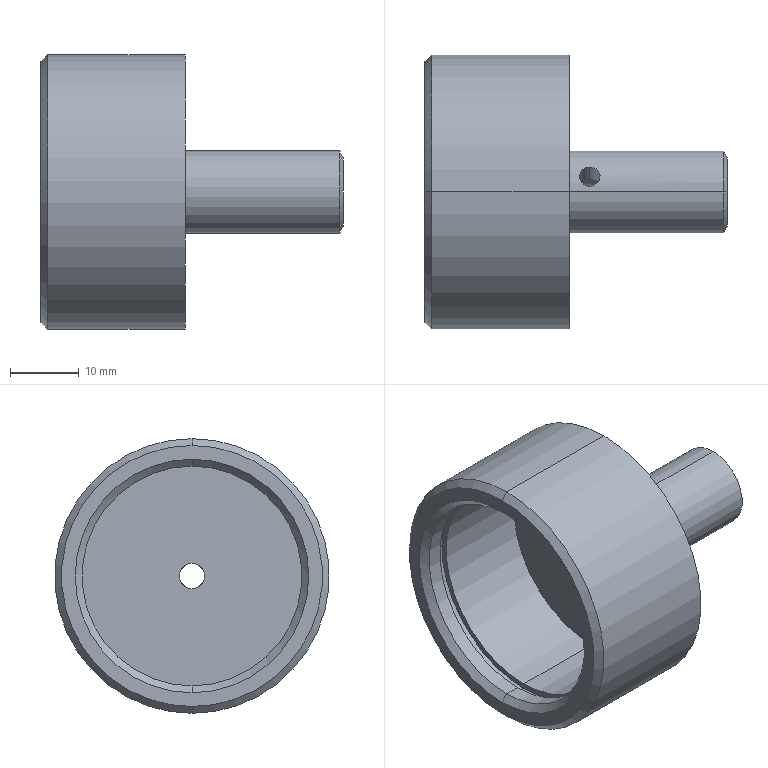Part | SolidWorks | features BaseBody 1 | 1 solid | 32 faces | box 44 x 40 x 40 mm | volume 13461 mm3 | cylinder 16 | cone 10 | plane 6 | commonest cylinder face diameters 32 x4 3 x2 3.691 x2 6 x2 12 x2 33.7 x2
STEP:
#1=CARTESIAN_POINT('',(226.,-84.,209.621));
#2=VERTEX_POINT('',#1);
#3=CARTESIAN_POINT('',(226.,-84.,169.621));
#4=VERTEX_POINT('',#3);
#5=CARTESIAN_POINT('',(226.,-84.,189.621));
#6=DIRECTION('',(-1.,0.,0.));
#7=DIRECTION('',(0.,0.,1.));
#8=AXIS2_PLACEMENT_3D('',#5,#6,#7);
#9=CIRCLE('',#8,20.);
#10=EDGE_CURVE('',#2,#4,#9,.T.);
#11=ORIENTED_EDGE('',*,*,#10,.T.);
#12=CARTESIAN_POINT('',(206.,-84.,169.621));
#13=VERTEX_POINT('',#12);
#14=CARTESIAN_POINT('',(205.,-84.,169.621));
#15=DIRECTION('',(-1.,0.,0.));
#16=VECTOR('',#15,1000.);
#17=LINE('',#14,#16);
#18=EDGE_CURVE('',#4,#13,#17,.T.);
#19=ORIENTED_EDGE('',*,*,#18,.T.);
#20=CARTESIAN_POINT('',(206.,-84.,209.621));
#21=VERTEX_POINT('',#20);
#22=CARTESIAN_POINT('',(206.,-84.,189.621));
#23=DIRECTION('',(1.,0.,0.));
#24=DIRECTION('',(0.,0.,1.));
#25=AXIS2_PLACEMENT_3D('',#22,#23,#24);
#26=CIRCLE('',#25,20.);
#27=EDGE_CURVE('',#13,#21,#26,.T.);
#28=ORIENTED_EDGE('',*,*,#27,.T.);
#29=CARTESIAN_POINT('',(205.,-84.,209.621));
#30=DIRECTION('',(-1.,0.,0.));
#31=VECTOR('',#30,1000.);
#32=LINE('',#29,#31);
#33=EDGE_CURVE('',#2,#21,#32,.T.);
#34=ORIENTED_EDGE('',*,*,#33,.F.);
#35=EDGE_LOOP('',(#11,#19,#28,#34));
#36=FACE_OUTER_BOUND('',#35,.T.);
#37=CARTESIAN_POINT('',(205.,-84.,189.621));
#38=DIRECTION('',(-1.,0.,0.));
#39=DIRECTION('',(0.,0.,1.));
#40=AXIS2_PLACEMENT_3D('',#37,#38,#39);
#41=CYLINDRICAL_SURFACE('',#40,20.);
#42=ADVANCED_FACE('',(#36),#41,.T.);
#43=CARTESIAN_POINT('',(205.,-84.,170.621));
#44=VERTEX_POINT('',#43);
#45=CARTESIAN_POINT('',(205.,-84.,208.621));
#46=VERTEX_POINT('',#45);
#47=CARTESIAN_POINT('',(205.,-84.,189.621));
#48=DIRECTION('',(1.,0.,0.));
#49=DIRECTION('',(0.,0.,-1.));
#50=AXIS2_PLACEMENT_3D('',#47,#48,#49);
#51=CIRCLE('',#50,19.);
#52=EDGE_CURVE('',#44,#46,#51,.T.);
#53=ORIENTED_EDGE('',*,*,#52,.T.);
#54=CARTESIAN_POINT('',(206.,-84.,209.621));
#55=DIRECTION('',(0.7071,0.,0.7071));
#56=VECTOR('',#55,1000.);
#57=LINE('',#54,#56);
#58=EDGE_CURVE('',#46,#21,#57,.T.);
#59=ORIENTED_EDGE('',*,*,#58,.T.);
#60=ORIENTED_EDGE('',*,*,#27,.F.);
#61=CARTESIAN_POINT('',(206.,-84.,169.621));
#62=DIRECTION('',(0.7071,0.,-0.7071));
#63=VECTOR('',#62,1000.);
#64=LINE('',#61,#63);
#65=EDGE_CURVE('',#44,#13,#64,.T.);
#66=ORIENTED_EDGE('',*,*,#65,.F.);
#67=EDGE_LOOP('',(#53,#59,#60,#66));
#68=FACE_OUTER_BOUND('',#67,.T.);
#69=CARTESIAN_POINT('',(206.,-84.,189.621));
#70=DIRECTION('',(1.,0.,0.));
#71=DIRECTION('',(0.,0.,-1.));
#72=AXIS2_PLACEMENT_3D('',#69,#70,#71);
#73=CONICAL_SURFACE('',#72,20.,0.7854);
#74=ADVANCED_FACE('',(#68),#73,.T.);
#75=CARTESIAN_POINT('',(229.,-80.395,194.418));
#76=VERTEX_POINT('',#75);
#77=CARTESIAN_POINT('',(229.,-83.168,195.563));
#78=VERTEX_POINT('',#77);
#79=CARTESIAN_POINT('',(229.,-80.395,194.418));
#80=CARTESIAN_POINT('',(229.099,-80.395,194.418));
#81=CARTESIAN_POINT('',(229.197,-80.403,194.424));
#82=CARTESIAN_POINT('',(229.389,-80.435,194.447));
#83=CARTESIAN_POINT('',(229.485,-80.459,194.465));
#84=CARTESIAN_POINT('',(229.666,-80.522,194.51));
#85=CARTESIAN_POINT('',(229.752,-80.56,194.538));
#86=CARTESIAN_POINT('',(229.915,-80.652,194.601));
#87=CARTESIAN_POINT('',(229.991,-80.706,194.636));
#88=CARTESIAN_POINT('',(230.198,-80.882,194.749));
#89=CARTESIAN_POINT('',(230.31,-81.027,194.836));
#90=CARTESIAN_POINT('',(230.46,-81.347,195.005));
#91=CARTESIAN_POINT('',(230.5,-81.525,195.09));
#92=CARTESIAN_POINT('',(230.5,-81.801,195.204));
#93=CARTESIAN_POINT('',(230.49,-81.892,195.239));
#94=CARTESIAN_POINT('',(230.452,-82.073,195.304));
#95=CARTESIAN_POINT('',(230.423,-82.164,195.334));
#96=CARTESIAN_POINT('',(230.348,-82.339,195.387));
#97=CARTESIAN_POINT('',(230.301,-82.422,195.41));
#98=CARTESIAN_POINT('',(230.193,-82.581,195.451));
#99=CARTESIAN_POINT('',(230.13,-82.657,195.469));
#100=CARTESIAN_POINT('',(229.923,-82.862,195.514));
#101=CARTESIAN_POINT('',(229.757,-82.974,195.533));
#102=CARTESIAN_POINT('',(229.396,-83.127,195.558));
#103=CARTESIAN_POINT('',(229.199,-83.168,195.563));
#104=CARTESIAN_POINT('',(229.,-83.168,195.563));
#105=B_SPLINE_CURVE_WITH_KNOTS('',3,(#79,#80,#81,#82,#83,#84,#85,#86,#87,#88,#89,#90,#91,#92,#93,#94,#95,#96,#97,#98,#99,#100,#101,#102,#103,#104),.UNSPECIFIED.,.F.,.F.,(4,2,2,2,2,2,2,2,2,2,2,2,4),(0.,0.0002941,0.0005882,0.0008822,0.001176,0.001764,0.002353,0.002647,0.002941,0.003235,0.003529,0.004117,0.004705),.UNSPECIFIED.);
#106=EDGE_CURVE('',#76,#78,#105,.T.);
#107=ORIENTED_EDGE('',*,*,#106,.T.);
#108=CARTESIAN_POINT('',(229.,-83.168,195.563));
#109=CARTESIAN_POINT('',(228.901,-83.168,195.563));
#110=CARTESIAN_POINT('',(228.803,-83.158,195.562));
#111=CARTESIAN_POINT('',(228.611,-83.119,195.556));
#112=CARTESIAN_POINT('',(228.515,-83.089,195.552));
#113=CARTESIAN_POINT('',(228.334,-83.013,195.539));
#114=CARTESIAN_POINT('',(228.248,-82.966,195.532));
#115=CARTESIAN_POINT('',(228.085,-82.857,195.511));
#116=CARTESIAN_POINT('',(228.009,-82.794,195.499));
#117=CARTESIAN_POINT('',(227.802,-82.589,195.454));
#118=CARTESIAN_POINT('',(227.69,-82.426,195.414));
#119=CARTESIAN_POINT('',(227.54,-82.079,195.308));
#120=CARTESIAN_POINT('',(227.5,-81.893,195.242));
#121=CARTESIAN_POINT('',(227.5,-81.617,195.128));
#122=CARTESIAN_POINT('',(227.51,-81.528,195.089));
#123=CARTESIAN_POINT('',(227.548,-81.354,195.007));
#124=CARTESIAN_POINT('',(227.577,-81.268,194.964));
#125=CARTESIAN_POINT('',(227.652,-81.107,194.878));
#126=CARTESIAN_POINT('',(227.699,-81.032,194.836));
#127=CARTESIAN_POINT('',(227.807,-80.89,194.753));
#128=CARTESIAN_POINT('',(227.87,-80.824,194.712));
#129=CARTESIAN_POINT('',(228.077,-80.647,194.599));
#130=CARTESIAN_POINT('',(228.243,-80.553,194.533));
#131=CARTESIAN_POINT('',(228.604,-80.428,194.443));
#132=CARTESIAN_POINT('',(228.801,-80.395,194.418));
#133=CARTESIAN_POINT('',(229.,-80.395,194.418));
#134=B_SPLINE_CURVE_WITH_KNOTS('',3,(#108,#109,#110,#111,#112,#113,#114,#115,#116,#117,#118,#119,#120,#121,#122,#123,#124,#125,#126,#127,#128,#129,#130,#131,#132,#133),.UNSPECIFIED.,.F.,.F.,(4,2,2,2,2,2,2,2,2,2,2,2,4),(-0.004705,-0.004411,-0.004117,-0.003823,-0.003529,-0.002941,-0.002352,-0.002058,-0.001764,-0.00147,-0.001176,-0.0005881,0.),.UNSPECIFIED.);
#135=EDGE_CURVE('',#78,#76,#134,.T.);
#136=ORIENTED_EDGE('',*,*,#135,.T.);
#137=EDGE_LOOP('',(#107,#136));
#138=FACE_BOUND('',#137,.T.);
#139=CARTESIAN_POINT('',(248.49,-84.,195.621));
#140=VERTEX_POINT('',#139);
#141=CARTESIAN_POINT('',(248.49,-84.,183.621));
#142=VERTEX_POINT('',#141);
#143=CARTESIAN_POINT('',(248.49,-84.,189.621));
#144=DIRECTION('',(-1.,0.,0.));
#145=DIRECTION('',(0.,0.,1.));
#146=AXIS2_PLACEMENT_3D('',#143,#144,#145);
#147=CIRCLE('',#146,6.);
#148=EDGE_CURVE('',#140,#142,#147,.T.);
#149=ORIENTED_EDGE('',*,*,#148,.T.);
#150=CARTESIAN_POINT('',(226.,-84.,183.621));
#151=VERTEX_POINT('',#150);
#152=CARTESIAN_POINT('',(205.,-84.,183.621));
#153=DIRECTION('',(-1.,0.,0.));
#154=VECTOR('',#153,1000.);
#155=LINE('',#152,#154);
#156=EDGE_CURVE('',#142,#151,#155,.T.);
#157=ORIENTED_EDGE('',*,*,#156,.T.);
#158=CARTESIAN_POINT('',(226.,-84.,195.621));
#159=VERTEX_POINT('',#158);
#160=CARTESIAN_POINT('',(226.,-84.,189.621));
#161=DIRECTION('',(1.,0.,0.));
#162=DIRECTION('',(0.,0.,1.));
#163=AXIS2_PLACEMENT_3D('',#160,#161,#162);
#164=CIRCLE('',#163,6.);
#165=EDGE_CURVE('',#151,#159,#164,.T.);
#166=ORIENTED_EDGE('',*,*,#165,.T.);
#167=CARTESIAN_POINT('',(205.,-84.,195.621));
#168=DIRECTION('',(-1.,0.,0.));
#169=VECTOR('',#168,1000.);
#170=LINE('',#167,#169);
#171=EDGE_CURVE('',#140,#159,#170,.T.);
#172=ORIENTED_EDGE('',*,*,#171,.F.);
#173=EDGE_LOOP('',(#149,#157,#166,#172));
#174=FACE_OUTER_BOUND('',#173,.T.);
#175=CARTESIAN_POINT('',(205.,-84.,189.621));
#176=DIRECTION('',(-1.,0.,0.));
#177=DIRECTION('',(0.,0.,1.));
#178=AXIS2_PLACEMENT_3D('',#175,#176,#177);
#179=CYLINDRICAL_SURFACE('',#178,6.);
#180=ADVANCED_FACE('',(#138,#174),#179,.T.);
#181=CARTESIAN_POINT('',(206.,-84.,173.621));
#182=VERTEX_POINT('',#181);
#183=CARTESIAN_POINT('',(206.,-84.,205.621));
#184=VERTEX_POINT('',#183);
#185=CARTESIAN_POINT('',(206.,-84.,189.621));
#186=DIRECTION('',(-1.,0.,0.));
#187=DIRECTION('',(0.,-0.3818,-0.9242));
#188=AXIS2_PLACEMENT_3D('',#185,#186,#187);
#189=CIRCLE('',#188,16.);
#190=EDGE_CURVE('',#182,#184,#189,.T.);
#191=ORIENTED_EDGE('',*,*,#190,.F.);
#192=CARTESIAN_POINT('',(205.,-84.,172.621));
#193=VERTEX_POINT('',#192);
#194=CARTESIAN_POINT('',(205.,-84.,172.621));
#195=DIRECTION('',(-0.7071,0.,-0.7071));
#196=VECTOR('',#195,1000.);
#197=LINE('',#194,#196);
#198=EDGE_CURVE('',#182,#193,#197,.T.);
#199=ORIENTED_EDGE('',*,*,#198,.T.);
#200=CARTESIAN_POINT('',(205.,-84.,206.621));
#201=VERTEX_POINT('',#200);
#202=CARTESIAN_POINT('',(205.,-84.,189.621));
#203=DIRECTION('',(-1.,0.,0.));
#204=DIRECTION('',(0.,0.,1.));
#205=AXIS2_PLACEMENT_3D('',#202,#203,#204);
#206=CIRCLE('',#205,17.);
#207=EDGE_CURVE('',#193,#201,#206,.T.);
#208=ORIENTED_EDGE('',*,*,#207,.T.);
#209=CARTESIAN_POINT('',(205.,-84.,206.621));
#210=DIRECTION('',(-0.7071,0.,0.7071));
#211=VECTOR('',#210,1000.);
#212=LINE('',#209,#211);
#213=EDGE_CURVE('',#184,#201,#212,.T.);
#214=ORIENTED_EDGE('',*,*,#213,.F.);
#215=EDGE_LOOP('',(#191,#199,#208,#214));
#216=FACE_OUTER_BOUND('',#215,.T.);
#217=CARTESIAN_POINT('',(205.,-84.,189.621));
#218=DIRECTION('',(-1.,0.,0.));
#219=DIRECTION('',(0.,0.,1.));
#220=AXIS2_PLACEMENT_3D('',#217,#218,#219);
#221=CONICAL_SURFACE('',#220,17.,0.7854);
#222=ADVANCED_FACE('',(#216),#221,.F.);
#223=CARTESIAN_POINT('',(249.,-84.,194.621));
#224=VERTEX_POINT('',#223);
#225=CARTESIAN_POINT('',(249.,-84.,184.621));
#226=VERTEX_POINT('',#225);
#227=CARTESIAN_POINT('',(249.,-84.,189.621));
#228=DIRECTION('',(-1.,0.,0.));
#229=DIRECTION('',(0.,0.,1.));
#230=AXIS2_PLACEMENT_3D('',#227,#228,#229);
#231=CIRCLE('',#230,5.);
#232=EDGE_CURVE('',#224,#226,#231,.T.);
#233=ORIENTED_EDGE('',*,*,#232,.T.);
#234=CARTESIAN_POINT('',(248.49,-84.,183.621));
#235=DIRECTION('',(-0.454,0.,-0.891));
#236=VECTOR('',#235,1000.);
#237=LINE('',#234,#236);
#238=EDGE_CURVE('',#226,#142,#237,.T.);
#239=ORIENTED_EDGE('',*,*,#238,.T.);
#240=ORIENTED_EDGE('',*,*,#148,.F.);
#241=CARTESIAN_POINT('',(248.49,-84.,195.621));
#242=DIRECTION('',(-0.454,0.,0.891));
#243=VECTOR('',#242,1000.);
#244=LINE('',#241,#243);
#245=EDGE_CURVE('',#224,#140,#244,.T.);
#246=ORIENTED_EDGE('',*,*,#245,.F.);
#247=EDGE_LOOP('',(#233,#239,#240,#246));
#248=FACE_OUTER_BOUND('',#247,.T.);
#249=CARTESIAN_POINT('',(248.49,-84.,189.621));
#250=DIRECTION('',(-1.,0.,0.));
#251=DIRECTION('',(0.,0.,1.));
#252=AXIS2_PLACEMENT_3D('',#249,#250,#251);
#253=CONICAL_SURFACE('',#252,6.,1.1);
#254=ADVANCED_FACE('',(#248),#253,.T.);
#255=ORIENTED_EDGE('',*,*,#135,.F.);
#256=CARTESIAN_POINT('',(229.,-84.976,191.187));
#257=VERTEX_POINT('',#256);
#258=CARTESIAN_POINT('',(229.,-77.749,208.678));
#259=DIRECTION('',(0.,-0.3818,-0.9242));
#260=VECTOR('',#259,1000.);
#261=LINE('',#258,#260);
#262=EDGE_CURVE('',#78,#257,#261,.T.);
#263=ORIENTED_EDGE('',*,*,#262,.T.);
#264=CARTESIAN_POINT('',(227.676,-84.,191.466));
#265=VERTEX_POINT('',#264);
#266=CARTESIAN_POINT('',(227.676,-84.,191.466));
#267=CARTESIAN_POINT('',(227.805,-84.262,191.466));
#268=CARTESIAN_POINT('',(227.99,-84.494,191.409));
#269=CARTESIAN_POINT('',(228.322,-84.758,191.306));
#270=CARTESIAN_POINT('',(228.442,-84.833,191.269));
#271=CARTESIAN_POINT('',(228.708,-84.943,191.208));
#272=CARTESIAN_POINT('',(228.852,-84.976,191.187));
#273=CARTESIAN_POINT('',(229.,-84.976,191.187));
#274=B_SPLINE_CURVE_WITH_KNOTS('',3,(#266,#267,#268,#269,#270,#271,#272,#273),.UNSPECIFIED.,.F.,.F.,(4,2,2,4),(0.005725,0.006597,0.007033,0.007468),.UNSPECIFIED.);
#275=EDGE_CURVE('',#265,#257,#274,.T.);
#276=ORIENTED_EDGE('',*,*,#275,.F.);
#277=CARTESIAN_POINT('',(229.,-82.203,190.042));
#278=VERTEX_POINT('',#277);
#279=CARTESIAN_POINT('',(229.,-82.203,190.042));
#280=CARTESIAN_POINT('',(228.863,-82.203,190.042));
#281=CARTESIAN_POINT('',(228.729,-82.21,190.074));
#282=CARTESIAN_POINT('',(228.48,-82.24,190.18));
#283=CARTESIAN_POINT('',(228.366,-82.263,190.25));
#284=CARTESIAN_POINT('',(228.154,-82.328,190.407));
#285=CARTESIAN_POINT('',(228.058,-82.37,190.493));
#286=CARTESIAN_POINT('',(227.883,-82.477,190.668));
#287=CARTESIAN_POINT('',(227.803,-82.543,190.759));
#288=CARTESIAN_POINT('',(227.601,-82.776,191.021));
#289=CARTESIAN_POINT('',(227.513,-82.988,191.188));
#290=CARTESIAN_POINT('',(227.496,-83.362,191.358));
#291=CARTESIAN_POINT('',(227.509,-83.491,191.4));
#292=CARTESIAN_POINT('',(227.569,-83.75,191.454));
#293=CARTESIAN_POINT('',(227.616,-83.878,191.466));
#294=CARTESIAN_POINT('',(227.676,-84.,191.466));
#295=B_SPLINE_CURVE_WITH_KNOTS('',3,(#279,#280,#281,#282,#283,#284,#285,#286,#287,#288,#289,#290,#291,#292,#293,#294),.UNSPECIFIED.,.F.,.F.,(4,2,2,2,2,2,2,4),(0.00249,0.002894,0.003298,0.003703,0.004107,0.004916,0.005321,0.005725),.UNSPECIFIED.);
#296=EDGE_CURVE('',#278,#265,#295,.T.);
#297=ORIENTED_EDGE('',*,*,#296,.F.);
#298=CARTESIAN_POINT('',(229.,-74.977,207.533));
#299=DIRECTION('',(0.,-0.3818,-0.9242));
#300=VECTOR('',#299,1000.);
#301=LINE('',#298,#300);
#302=EDGE_CURVE('',#76,#278,#301,.T.);
#303=ORIENTED_EDGE('',*,*,#302,.F.);
#304=EDGE_LOOP('',(#255,#263,#276,#297,#303));
#305=FACE_OUTER_BOUND('',#304,.T.);
#306=CARTESIAN_POINT('',(229.,-76.363,208.106));
#307=DIRECTION('',(0.,-0.3818,-0.9242));
#308=DIRECTION('',(0.,0.9242,-0.3818));
#309=AXIS2_PLACEMENT_3D('',#306,#307,#308);
#310=CYLINDRICAL_SURFACE('',#309,1.5);
#311=ADVANCED_FACE('',(#305),#310,.F.);
#312=CARTESIAN_POINT('',(208.2,-84.,173.621));
#313=VERTEX_POINT('',#312);
#314=CARTESIAN_POINT('',(208.2,-84.,205.621));
#315=VERTEX_POINT('',#314);
#316=CARTESIAN_POINT('',(208.2,-84.,189.621));
#317=DIRECTION('',(-1.,0.,0.));
#318=DIRECTION('',(0.,0.,1.));
#319=AXIS2_PLACEMENT_3D('',#316,#317,#318);
#320=CIRCLE('',#319,16.);
#321=EDGE_CURVE('',#313,#315,#320,.T.);
#322=ORIENTED_EDGE('',*,*,#321,.F.);
#323=CARTESIAN_POINT('',(223.5,-84.,173.621));
#324=DIRECTION('',(-1.,0.,0.));
#325=VECTOR('',#324,1000.);
#326=LINE('',#323,#325);
#327=EDGE_CURVE('',#313,#182,#326,.T.);
#328=ORIENTED_EDGE('',*,*,#327,.T.);
#329=ORIENTED_EDGE('',*,*,#190,.T.);
#330=CARTESIAN_POINT('',(223.5,-84.,205.621));
#331=DIRECTION('',(-1.,0.,0.));
#332=VECTOR('',#331,1000.);
#333=LINE('',#330,#332);
#334=EDGE_CURVE('',#315,#184,#333,.T.);
#335=ORIENTED_EDGE('',*,*,#334,.F.);
#336=EDGE_LOOP('',(#322,#328,#329,#335));
#337=FACE_OUTER_BOUND('',#336,.T.);
#338=CARTESIAN_POINT('',(223.5,-84.,189.621));
#339=DIRECTION('',(-1.,0.,0.));
#340=DIRECTION('',(0.,0.,1.));
#341=AXIS2_PLACEMENT_3D('',#338,#339,#340);
#342=CYLINDRICAL_SURFACE('',#341,16.);
#343=ADVANCED_FACE('',(#337),#342,.F.);
#344=CARTESIAN_POINT('',(223.5,-84.,191.466));
#345=VERTEX_POINT('',#344);
#346=CARTESIAN_POINT('',(223.5,-84.,187.776));
#347=VERTEX_POINT('',#346);
#348=CARTESIAN_POINT('',(223.5,-84.,189.621));
#349=DIRECTION('',(1.,0.,0.));
#350=DIRECTION('',(0.,0.,-1.));
#351=AXIS2_PLACEMENT_3D('',#348,#349,#350);
#352=CIRCLE('',#351,1.845);
#353=EDGE_CURVE('',#345,#347,#352,.T.);
#354=ORIENTED_EDGE('',*,*,#353,.F.);
#355=CARTESIAN_POINT('',(214.75,-84.,191.466));
#356=DIRECTION('',(1.,0.,0.));
#357=VECTOR('',#356,1000.);
#358=LINE('',#355,#357);
#359=EDGE_CURVE('',#345,#265,#358,.T.);
#360=ORIENTED_EDGE('',*,*,#359,.T.);
#361=ORIENTED_EDGE('',*,*,#275,.T.);
#362=CARTESIAN_POINT('',(230.324,-84.,191.466));
#363=VERTEX_POINT('',#362);
#364=CARTESIAN_POINT('',(229.,-84.976,191.187));
#365=CARTESIAN_POINT('',(229.148,-84.976,191.187));
#366=CARTESIAN_POINT('',(229.292,-84.943,191.208));
#367=CARTESIAN_POINT('',(229.557,-84.834,191.268));
#368=CARTESIAN_POINT('',(229.678,-84.758,191.306));
#369=CARTESIAN_POINT('',(229.9,-84.581,191.375));
#370=CARTESIAN_POINT('',(230.,-84.48,191.406));
#371=CARTESIAN_POINT('',(230.18,-84.255,191.452));
#372=CARTESIAN_POINT('',(230.26,-84.131,191.466));
#373=CARTESIAN_POINT('',(230.324,-84.,191.466));
#374=B_SPLINE_CURVE_WITH_KNOTS('',3,(#364,#365,#366,#367,#368,#369,#370,#371,#372,#373),.UNSPECIFIED.,.F.,.F.,(4,2,2,2,4),(-0.002489,-0.002053,-0.001617,-0.00118,-0.0007441),.UNSPECIFIED.);
#375=EDGE_CURVE('',#257,#363,#374,.T.);
#376=ORIENTED_EDGE('',*,*,#375,.T.);
#377=CARTESIAN_POINT('',(242.134,-84.,191.466));
#378=VERTEX_POINT('',#377);
#379=CARTESIAN_POINT('',(214.75,-84.,191.466));
#380=DIRECTION('',(1.,0.,0.));
#381=VECTOR('',#380,1000.);
#382=LINE('',#379,#381);
#383=EDGE_CURVE('',#363,#378,#382,.T.);
#384=ORIENTED_EDGE('',*,*,#383,.T.);
#385=CARTESIAN_POINT('',(242.134,-85.845,189.621));
#386=VERTEX_POINT('',#385);
#387=CARTESIAN_POINT('',(242.134,-84.,189.621));
#388=DIRECTION('',(-1.,0.,0.));
#389=DIRECTION('',(0.,0.,-1.));
#390=AXIS2_PLACEMENT_3D('',#387,#388,#389);
#391=CIRCLE('',#390,1.845);
#392=EDGE_CURVE('',#386,#378,#391,.T.);
#393=ORIENTED_EDGE('',*,*,#392,.F.);
#394=CARTESIAN_POINT('',(242.134,-84.,187.776));
#395=VERTEX_POINT('',#394);
#396=CARTESIAN_POINT('',(242.134,-84.,189.621));
#397=DIRECTION('',(-1.,0.,0.));
#398=DIRECTION('',(0.,0.,-1.));
#399=AXIS2_PLACEMENT_3D('',#396,#397,#398);
#400=CIRCLE('',#399,1.845);
#401=EDGE_CURVE('',#395,#386,#400,.T.);
#402=ORIENTED_EDGE('',*,*,#401,.F.);
#403=CARTESIAN_POINT('',(214.75,-84.,187.776));
#404=DIRECTION('',(1.,0.,0.));
#405=VECTOR('',#404,1000.);
#406=LINE('',#403,#405);
#407=EDGE_CURVE('',#347,#395,#406,.T.);
#408=ORIENTED_EDGE('',*,*,#407,.F.);
#409=EDGE_LOOP('',(#354,#360,#361,#376,#384,#393,#402,#408));
#410=FACE_OUTER_BOUND('',#409,.T.);
#411=CARTESIAN_POINT('',(214.75,-84.,189.621));
#412=DIRECTION('',(1.,0.,0.));
#413=DIRECTION('',(0.,0.,-1.));
#414=AXIS2_PLACEMENT_3D('',#411,#412,#413);
#415=CYLINDRICAL_SURFACE('',#414,1.845);
#416=ADVANCED_FACE('',(#410),#415,.F.);
#417=CARTESIAN_POINT('',(248.,-87.,189.621));
#418=VERTEX_POINT('',#417);
#419=CARTESIAN_POINT('',(248.,-84.,186.621));
#420=VERTEX_POINT('',#419);
#421=CARTESIAN_POINT('',(248.,-84.,189.621));
#422=DIRECTION('',(1.,0.,0.));
#423=DIRECTION('',(0.,0.3818,0.9242));
#424=AXIS2_PLACEMENT_3D('',#421,#422,#423);
#425=CIRCLE('',#424,3.);
#426=EDGE_CURVE('',#418,#420,#425,.T.);
#427=ORIENTED_EDGE('',*,*,#426,.F.);
#428=CARTESIAN_POINT('',(249.,-88.,189.621));
#429=VERTEX_POINT('',#428);
#430=CARTESIAN_POINT('',(249.,-88.,189.621));
#431=DIRECTION('',(0.7071,-0.7071,0.));
#432=VECTOR('',#431,1000.);
#433=LINE('',#430,#432);
#434=EDGE_CURVE('',#418,#429,#433,.T.);
#435=ORIENTED_EDGE('',*,*,#434,.T.);
#436=CARTESIAN_POINT('',(249.,-80.,189.621));
#437=VERTEX_POINT('',#436);
#438=CARTESIAN_POINT('',(249.,-84.,189.621));
#439=DIRECTION('',(1.,0.,0.));
#440=DIRECTION('',(0.,1.,0.));
#441=AXIS2_PLACEMENT_3D('',#438,#439,#440);
#442=CIRCLE('',#441,4.);
#443=EDGE_CURVE('',#429,#437,#442,.T.);
#444=ORIENTED_EDGE('',*,*,#443,.T.);
#445=CARTESIAN_POINT('',(248.,-81.,189.621));
#446=VERTEX_POINT('',#445);
#447=CARTESIAN_POINT('',(249.,-80.,189.621));
#448=DIRECTION('',(0.7071,0.7071,0.));
#449=VECTOR('',#448,1000.);
#450=LINE('',#447,#449);
#451=EDGE_CURVE('',#446,#437,#450,.T.);
#452=ORIENTED_EDGE('',*,*,#451,.F.);
#453=CARTESIAN_POINT('',(248.,-84.,189.621));
#454=DIRECTION('',(1.,0.,0.));
#455=DIRECTION('',(0.,0.3818,0.9242));
#456=AXIS2_PLACEMENT_3D('',#453,#454,#455);
#457=CIRCLE('',#456,3.);
#458=EDGE_CURVE('',#420,#446,#457,.T.);
#459=ORIENTED_EDGE('',*,*,#458,.F.);
#460=EDGE_LOOP('',(#427,#435,#444,#452,#459));
#461=FACE_OUTER_BOUND('',#460,.T.);
#462=CARTESIAN_POINT('',(249.,-84.,189.621));
#463=DIRECTION('',(1.,0.,0.));
#464=DIRECTION('',(0.,1.,0.));
#465=AXIS2_PLACEMENT_3D('',#462,#463,#464);
#466=CONICAL_SURFACE('',#465,4.,0.7854);
#467=ADVANCED_FACE('',(#461),#466,.F.);
#468=CARTESIAN_POINT('',(242.134,-82.155,189.621));
#469=VERTEX_POINT('',#468);
#470=CARTESIAN_POINT('',(242.134,-84.,189.621));
#471=DIRECTION('',(-1.,0.,0.));
#472=DIRECTION('',(0.,0.,-1.));
#473=AXIS2_PLACEMENT_3D('',#470,#471,#472);
#474=CIRCLE('',#473,1.845);
#475=EDGE_CURVE('',#469,#395,#474,.T.);
#476=ORIENTED_EDGE('',*,*,#475,.T.);
#477=ORIENTED_EDGE('',*,*,#401,.T.);
#478=CARTESIAN_POINT('',(244.134,-87.,189.621));
#479=VERTEX_POINT('',#478);
#480=CARTESIAN_POINT('',(244.134,-87.,189.621));
#481=DIRECTION('',(0.866,-0.5,0.));
#482=VECTOR('',#481,1000.);
#483=LINE('',#480,#482);
#484=EDGE_CURVE('',#386,#479,#483,.T.);
#485=ORIENTED_EDGE('',*,*,#484,.T.);
#486=CARTESIAN_POINT('',(244.134,-84.,186.621));
#487=VERTEX_POINT('',#486);
#488=CARTESIAN_POINT('',(244.134,-84.,189.621));
#489=DIRECTION('',(-1.,0.,0.));
#490=DIRECTION('',(0.,-0.3818,-0.9242));
#491=AXIS2_PLACEMENT_3D('',#488,#489,#490);
#492=CIRCLE('',#491,3.);
#493=EDGE_CURVE('',#487,#479,#492,.T.);
#494=ORIENTED_EDGE('',*,*,#493,.F.);
#495=CARTESIAN_POINT('',(244.134,-81.,189.621));
#496=VERTEX_POINT('',#495);
#497=CARTESIAN_POINT('',(244.134,-84.,189.621));
#498=DIRECTION('',(-1.,0.,0.));
#499=DIRECTION('',(0.,-0.3818,-0.9242));
#500=AXIS2_PLACEMENT_3D('',#497,#498,#499);
#501=CIRCLE('',#500,3.);
#502=EDGE_CURVE('',#496,#487,#501,.T.);
#503=ORIENTED_EDGE('',*,*,#502,.F.);
#504=CARTESIAN_POINT('',(244.134,-81.,189.621));
#505=DIRECTION('',(0.866,0.5,0.));
#506=VECTOR('',#505,1000.);
#507=LINE('',#504,#506);
#508=EDGE_CURVE('',#469,#496,#507,.T.);
#509=ORIENTED_EDGE('',*,*,#508,.F.);
#510=EDGE_LOOP('',(#476,#477,#485,#494,#503,#509));
#511=FACE_OUTER_BOUND('',#510,.T.);
#512=CARTESIAN_POINT('',(244.134,-84.,189.621));
#513=DIRECTION('',(1.,0.,0.));
#514=DIRECTION('',(0.,1.,0.));
#515=AXIS2_PLACEMENT_3D('',#512,#513,#514);
#516=CONICAL_SURFACE('',#515,3.,0.5236);
#517=ADVANCED_FACE('',(#511),#516,.F.);
#518=CARTESIAN_POINT('',(208.2,-83.982,172.815));
#519=VERTEX_POINT('',#518);
#520=CARTESIAN_POINT('',(208.2,-83.982,206.515));
#521=VERTEX_POINT('',#520);
#522=CARTESIAN_POINT('',(208.2,-83.982,189.665));
#523=DIRECTION('',(-1.,0.,0.));
#524=DIRECTION('',(0.,0.,-1.));
#525=AXIS2_PLACEMENT_3D('',#522,#523,#524);
#526=CIRCLE('',#525,16.85);
#527=EDGE_CURVE('',#519,#521,#526,.T.);
#528=ORIENTED_EDGE('',*,*,#527,.T.);
#529=CARTESIAN_POINT('',(209.5,-83.982,206.515));
#530=VERTEX_POINT('',#529);
#531=CARTESIAN_POINT('',(209.5,-83.982,206.515));
#532=DIRECTION('',(1.,0.,0.));
#533=VECTOR('',#532,1000.);
#534=LINE('',#531,#533);
#535=EDGE_CURVE('',#521,#530,#534,.T.);
#536=ORIENTED_EDGE('',*,*,#535,.T.);
#537=CARTESIAN_POINT('',(209.5,-83.982,172.815));
#538=VERTEX_POINT('',#537);
#539=CARTESIAN_POINT('',(209.5,-83.982,189.665));
#540=DIRECTION('',(-1.,0.,0.));
#541=DIRECTION('',(0.,0.,-1.));
#542=AXIS2_PLACEMENT_3D('',#539,#540,#541);
#543=CIRCLE('',#542,16.85);
#544=EDGE_CURVE('',#538,#530,#543,.T.);
#545=ORIENTED_EDGE('',*,*,#544,.F.);
#546=CARTESIAN_POINT('',(209.5,-83.982,172.815));
#547=DIRECTION('',(1.,0.,0.));
#548=VECTOR('',#547,1000.);
#549=LINE('',#546,#548);
#550=EDGE_CURVE('',#519,#538,#549,.T.);
#551=ORIENTED_EDGE('',*,*,#550,.F.);
#552=EDGE_LOOP('',(#528,#536,#545,#551));
#553=FACE_OUTER_BOUND('',#552,.T.);
#554=CARTESIAN_POINT('',(209.5,-83.982,189.665));
#555=DIRECTION('',(1.,0.,0.));
#556=DIRECTION('',(0.,0.,-1.));
#557=AXIS2_PLACEMENT_3D('',#554,#555,#556);
#558=CYLINDRICAL_SURFACE('',#557,16.85);
#559=ADVANCED_FACE('',(#553),#558,.F.);
#560=ORIENTED_EDGE('',*,*,#493,.T.);
#561=CARTESIAN_POINT('',(244.134,-84.,192.621));
#562=VERTEX_POINT('',#561);
#563=CARTESIAN_POINT('',(244.134,-84.,189.621));
#564=DIRECTION('',(-1.,0.,0.));
#565=DIRECTION('',(0.,-0.3818,-0.9242));
#566=AXIS2_PLACEMENT_3D('',#563,#564,#565);
#567=CIRCLE('',#566,3.);
#568=EDGE_CURVE('',#479,#562,#567,.T.);
#569=ORIENTED_EDGE('',*,*,#568,.T.);
#570=CARTESIAN_POINT('',(248.,-84.,192.621));
#571=VERTEX_POINT('',#570);
#572=CARTESIAN_POINT('',(242.134,-84.,192.621));
#573=DIRECTION('',(1.,0.,0.));
#574=VECTOR('',#573,1000.);
#575=LINE('',#572,#574);
#576=EDGE_CURVE('',#562,#571,#575,.T.);
#577=ORIENTED_EDGE('',*,*,#576,.T.);
#578=CARTESIAN_POINT('',(248.,-84.,189.621));
#579=DIRECTION('',(1.,0.,0.));
#580=DIRECTION('',(0.,0.3818,0.9242));
#581=AXIS2_PLACEMENT_3D('',#578,#579,#580);
#582=CIRCLE('',#581,3.);
#583=EDGE_CURVE('',#571,#418,#582,.T.);
#584=ORIENTED_EDGE('',*,*,#583,.T.);
#585=ORIENTED_EDGE('',*,*,#426,.T.);
#586=CARTESIAN_POINT('',(242.134,-84.,186.621));
#587=DIRECTION('',(1.,0.,0.));
#588=VECTOR('',#587,1000.);
#589=LINE('',#586,#588);
#590=EDGE_CURVE('',#487,#420,#589,.T.);
#591=ORIENTED_EDGE('',*,*,#590,.F.);
#592=EDGE_LOOP('',(#560,#569,#577,#584,#585,#591));
#593=FACE_OUTER_BOUND('',#592,.T.);
#594=CARTESIAN_POINT('',(242.134,-84.,189.621));
#595=DIRECTION('',(1.,0.,0.));
#596=DIRECTION('',(0.,0.,-1.));
#597=AXIS2_PLACEMENT_3D('',#594,#595,#596);
#598=CYLINDRICAL_SURFACE('',#597,3.);
#599=ADVANCED_FACE('',(#593),#598,.F.);
#600=CARTESIAN_POINT('',(223.5,-84.,173.621));
#601=VERTEX_POINT('',#600);
#602=CARTESIAN_POINT('',(223.5,-84.,205.621));
#603=VERTEX_POINT('',#602);
#604=CARTESIAN_POINT('',(223.5,-84.,189.621));
#605=DIRECTION('',(-1.,0.,0.));
#606=DIRECTION('',(0.,0.,1.));
#607=AXIS2_PLACEMENT_3D('',#604,#605,#606);
#608=CIRCLE('',#607,16.);
#609=EDGE_CURVE('',#601,#603,#608,.T.);
#610=ORIENTED_EDGE('',*,*,#609,.F.);
#611=CARTESIAN_POINT('',(209.5,-84.,173.621));
#612=VERTEX_POINT('',#611);
#613=CARTESIAN_POINT('',(223.5,-84.,173.621));
#614=DIRECTION('',(-1.,0.,0.));
#615=VECTOR('',#614,1000.);
#616=LINE('',#613,#615);
#617=EDGE_CURVE('',#601,#612,#616,.T.);
#618=ORIENTED_EDGE('',*,*,#617,.T.);
#619=CARTESIAN_POINT('',(209.5,-84.,205.621));
#620=VERTEX_POINT('',#619);
#621=CARTESIAN_POINT('',(209.5,-84.,189.621));
#622=DIRECTION('',(1.,0.,0.));
#623=DIRECTION('',(0.,0.,1.));
#624=AXIS2_PLACEMENT_3D('',#621,#622,#623);
#625=CIRCLE('',#624,16.);
#626=EDGE_CURVE('',#620,#612,#625,.T.);
#627=ORIENTED_EDGE('',*,*,#626,.F.);
#628=CARTESIAN_POINT('',(223.5,-84.,205.621));
#629=DIRECTION('',(-1.,0.,0.));
#630=VECTOR('',#629,1000.);
#631=LINE('',#628,#630);
#632=EDGE_CURVE('',#603,#620,#631,.T.);
#633=ORIENTED_EDGE('',*,*,#632,.F.);
#634=EDGE_LOOP('',(#610,#618,#627,#633));
#635=FACE_OUTER_BOUND('',#634,.T.);
#636=CARTESIAN_POINT('',(223.5,-84.,189.621));
#637=DIRECTION('',(-1.,0.,0.));
#638=DIRECTION('',(0.,0.,1.));
#639=AXIS2_PLACEMENT_3D('',#636,#637,#638);
#640=CYLINDRICAL_SURFACE('',#639,16.);
#641=ADVANCED_FACE('',(#635),#640,.F.);
#642=ORIENTED_EDGE('',*,*,#18,.F.);
#643=CARTESIAN_POINT('',(226.,-84.,189.621));
#644=DIRECTION('',(-1.,0.,0.));
#645=DIRECTION('',(0.,0.,1.));
#646=AXIS2_PLACEMENT_3D('',#643,#644,#645);
#647=CIRCLE('',#646,20.);
#648=EDGE_CURVE('',#4,#2,#647,.T.);
#649=ORIENTED_EDGE('',*,*,#648,.T.);
#650=ORIENTED_EDGE('',*,*,#33,.T.);
#651=CARTESIAN_POINT('',(206.,-84.,189.621));
#652=DIRECTION('',(1.,0.,0.));
#653=DIRECTION('',(0.,0.,1.));
#654=AXIS2_PLACEMENT_3D('',#651,#652,#653);
#655=CIRCLE('',#654,20.);
#656=EDGE_CURVE('',#21,#13,#655,.T.);
#657=ORIENTED_EDGE('',*,*,#656,.T.);
#658=EDGE_LOOP('',(#642,#649,#650,#657));
#659=FACE_OUTER_BOUND('',#658,.T.);
#660=CARTESIAN_POINT('',(205.,-84.,189.621));
#661=DIRECTION('',(-1.,0.,0.));
#662=DIRECTION('',(0.,0.,1.));
#663=AXIS2_PLACEMENT_3D('',#660,#661,#662);
#664=CYLINDRICAL_SURFACE('',#663,20.);
#665=ADVANCED_FACE('',(#659),#664,.T.);
#666=ORIENTED_EDGE('',*,*,#58,.F.);
#667=CARTESIAN_POINT('',(205.,-84.,189.621));
#668=DIRECTION('',(1.,0.,0.));
#669=DIRECTION('',(0.,0.,-1.));
#670=AXIS2_PLACEMENT_3D('',#667,#668,#669);
#671=CIRCLE('',#670,19.);
#672=EDGE_CURVE('',#46,#44,#671,.T.);
#673=ORIENTED_EDGE('',*,*,#672,.T.);
#674=ORIENTED_EDGE('',*,*,#65,.T.);
#675=ORIENTED_EDGE('',*,*,#656,.F.);
#676=EDGE_LOOP('',(#666,#673,#674,#675));
#677=FACE_OUTER_BOUND('',#676,.T.);
#678=CARTESIAN_POINT('',(206.,-84.,189.621));
#679=DIRECTION('',(1.,0.,0.));
#680=DIRECTION('',(0.,0.,-1.));
#681=AXIS2_PLACEMENT_3D('',#678,#679,#680);
#682=CONICAL_SURFACE('',#681,20.,0.7854);
#683=ADVANCED_FACE('',(#677),#682,.T.);
#684=CARTESIAN_POINT('',(226.,-84.,189.621));
#685=DIRECTION('',(1.,0.,0.));
#686=DIRECTION('',(0.,0.,1.));
#687=AXIS2_PLACEMENT_3D('',#684,#685,#686);
#688=CIRCLE('',#687,6.);
#689=EDGE_CURVE('',#159,#151,#688,.T.);
#690=ORIENTED_EDGE('',*,*,#689,.F.);
#691=ORIENTED_EDGE('',*,*,#165,.F.);
#692=EDGE_LOOP('',(#690,#691));
#693=FACE_BOUND('',#692,.T.);
#694=ORIENTED_EDGE('',*,*,#10,.F.);
#695=ORIENTED_EDGE('',*,*,#648,.F.);
#696=EDGE_LOOP('',(#694,#695));
#697=FACE_OUTER_BOUND('',#696,.T.);
#698=CARTESIAN_POINT('',(226.,-89.545,191.912));
#699=DIRECTION('',(-1.,0.,0.));
#700=DIRECTION('',(0.,0.,1.));
#701=AXIS2_PLACEMENT_3D('',#698,#699,#700);
#702=PLANE('',#701);
#703=ADVANCED_FACE('',(#693,#697),#702,.F.);
#704=ORIENTED_EDGE('',*,*,#52,.F.);
#705=ORIENTED_EDGE('',*,*,#672,.F.);
#706=EDGE_LOOP('',(#704,#705));
#707=FACE_OUTER_BOUND('',#706,.T.);
#708=CARTESIAN_POINT('',(205.,-84.,189.621));
#709=DIRECTION('',(-1.,0.,0.));
#710=DIRECTION('',(0.,0.,1.));
#711=AXIS2_PLACEMENT_3D('',#708,#709,#710);
#712=CIRCLE('',#711,17.);
#713=EDGE_CURVE('',#201,#193,#712,.T.);
#714=ORIENTED_EDGE('',*,*,#713,.F.);
#715=ORIENTED_EDGE('',*,*,#207,.F.);
#716=EDGE_LOOP('',(#714,#715));
#717=FACE_BOUND('',#716,.T.);
#718=CARTESIAN_POINT('',(205.,-102.484,197.258));
#719=DIRECTION('',(1.,0.,0.));
#720=DIRECTION('',(0.,0.,-1.));
#721=AXIS2_PLACEMENT_3D('',#718,#719,#720);
#722=PLANE('',#721);
#723=ADVANCED_FACE('',(#707,#717),#722,.F.);
#724=ORIENTED_EDGE('',*,*,#156,.F.);
#725=CARTESIAN_POINT('',(248.49,-84.,189.621));
#726=DIRECTION('',(-1.,0.,0.));
#727=DIRECTION('',(0.,0.,1.));
#728=AXIS2_PLACEMENT_3D('',#725,#726,#727);
#729=CIRCLE('',#728,6.);
#730=EDGE_CURVE('',#142,#140,#729,.T.);
#731=ORIENTED_EDGE('',*,*,#730,.T.);
#732=ORIENTED_EDGE('',*,*,#171,.T.);
#733=ORIENTED_EDGE('',*,*,#689,.T.);
#734=EDGE_LOOP('',(#724,#731,#732,#733));
#735=FACE_OUTER_BOUND('',#734,.T.);
#736=CARTESIAN_POINT('',(205.,-84.,189.621));
#737=DIRECTION('',(-1.,0.,0.));
#738=DIRECTION('',(0.,0.,1.));
#739=AXIS2_PLACEMENT_3D('',#736,#737,#738);
#740=CYLINDRICAL_SURFACE('',#739,6.);
#741=ADVANCED_FACE('',(#735),#740,.T.);
#742=ORIENTED_EDGE('',*,*,#198,.F.);
#743=CARTESIAN_POINT('',(206.,-84.,189.621));
#744=DIRECTION('',(-1.,0.,0.));
#745=DIRECTION('',(0.,-0.3818,-0.9242));
#746=AXIS2_PLACEMENT_3D('',#743,#744,#745);
#747=CIRCLE('',#746,16.);
#748=EDGE_CURVE('',#184,#182,#747,.T.);
#749=ORIENTED_EDGE('',*,*,#748,.F.);
#750=ORIENTED_EDGE('',*,*,#213,.T.);
#751=ORIENTED_EDGE('',*,*,#713,.T.);
#752=EDGE_LOOP('',(#742,#749,#750,#751));
#753=FACE_OUTER_BOUND('',#752,.T.);
#754=CARTESIAN_POINT('',(205.,-84.,189.621));
#755=DIRECTION('',(-1.,0.,0.));
#756=DIRECTION('',(0.,0.,1.));
#757=AXIS2_PLACEMENT_3D('',#754,#755,#756);
#758=CONICAL_SURFACE('',#757,17.,0.7854);
#759=ADVANCED_FACE('',(#753),#758,.F.);
#760=ORIENTED_EDGE('',*,*,#238,.F.);
#761=CARTESIAN_POINT('',(249.,-84.,189.621));
#762=DIRECTION('',(-1.,0.,0.));
#763=DIRECTION('',(0.,0.,1.));
#764=AXIS2_PLACEMENT_3D('',#761,#762,#763);
#765=CIRCLE('',#764,5.);
#766=EDGE_CURVE('',#226,#224,#765,.T.);
#767=ORIENTED_EDGE('',*,*,#766,.T.);
#768=ORIENTED_EDGE('',*,*,#245,.T.);
#769=ORIENTED_EDGE('',*,*,#730,.F.);
#770=EDGE_LOOP('',(#760,#767,#768,#769));
#771=FACE_OUTER_BOUND('',#770,.T.);
#772=CARTESIAN_POINT('',(248.49,-84.,189.621));
#773=DIRECTION('',(-1.,0.,0.));
#774=DIRECTION('',(0.,0.,1.));
#775=AXIS2_PLACEMENT_3D('',#772,#773,#774);
#776=CONICAL_SURFACE('',#775,6.,1.1);
#777=ADVANCED_FACE('',(#771),#776,.T.);
#778=ORIENTED_EDGE('',*,*,#262,.F.);
#779=ORIENTED_EDGE('',*,*,#106,.F.);
#780=ORIENTED_EDGE('',*,*,#302,.T.);
#781=CARTESIAN_POINT('',(230.324,-84.,191.466));
#782=CARTESIAN_POINT('',(230.384,-83.879,191.466));
#783=CARTESIAN_POINT('',(230.431,-83.749,191.454));
#784=CARTESIAN_POINT('',(230.491,-83.492,191.4));
#785=CARTESIAN_POINT('',(230.504,-83.359,191.357));
#786=CARTESIAN_POINT('',(230.493,-83.112,191.244));
#787=CARTESIAN_POINT('',(230.469,-82.997,191.176));
#788=CARTESIAN_POINT('',(230.387,-82.789,191.02));
#789=CARTESIAN_POINT('',(230.332,-82.699,190.935));
#790=CARTESIAN_POINT('',(230.196,-82.542,190.758));
#791=CARTESIAN_POINT('',(230.118,-82.478,190.669));
#792=CARTESIAN_POINT('',(229.943,-82.371,190.493));
#793=CARTESIAN_POINT('',(229.845,-82.328,190.407));
#794=CARTESIAN_POINT('',(229.635,-82.264,190.251));
#795=CARTESIAN_POINT('',(229.521,-82.241,190.18));
#796=CARTESIAN_POINT('',(229.272,-82.21,190.074));
#797=CARTESIAN_POINT('',(229.137,-82.203,190.042));
#798=CARTESIAN_POINT('',(229.,-82.203,190.042));
#799=B_SPLINE_CURVE_WITH_KNOTS('',3,(#781,#782,#783,#784,#785,#786,#787,#788,#789,#790,#791,#792,#793,#794,#795,#796,#797,#798),.UNSPECIFIED.,.F.,.F.,(4,2,2,2,2,2,2,2,4),(-0.0007441,-0.0003399,0.0000643,0.0004685,0.0008727,0.001277,0.001681,0.002085,0.00249),.UNSPECIFIED.);
#800=EDGE_CURVE('',#363,#278,#799,.T.);
#801=ORIENTED_EDGE('',*,*,#800,.F.);
#802=ORIENTED_EDGE('',*,*,#375,.F.);
#803=EDGE_LOOP('',(#778,#779,#780,#801,#802));
#804=FACE_OUTER_BOUND('',#803,.T.);
#805=CARTESIAN_POINT('',(229.,-76.363,208.106));
#806=DIRECTION('',(0.,-0.3818,-0.9242));
#807=DIRECTION('',(0.,0.9242,-0.3818));
#808=AXIS2_PLACEMENT_3D('',#805,#806,#807);
#809=CYLINDRICAL_SURFACE('',#808,1.5);
#810=ADVANCED_FACE('',(#804),#809,.F.);
#811=ORIENTED_EDGE('',*,*,#327,.F.);
#812=CARTESIAN_POINT('',(208.2,-84.,189.621));
#813=DIRECTION('',(-1.,0.,0.));
#814=DIRECTION('',(0.,0.,1.));
#815=AXIS2_PLACEMENT_3D('',#812,#813,#814);
#816=CIRCLE('',#815,16.);
#817=EDGE_CURVE('',#315,#313,#816,.T.);
#818=ORIENTED_EDGE('',*,*,#817,.F.);
#819=ORIENTED_EDGE('',*,*,#334,.T.);
#820=ORIENTED_EDGE('',*,*,#748,.T.);
#821=EDGE_LOOP('',(#811,#818,#819,#820));
#822=FACE_OUTER_BOUND('',#821,.T.);
#823=CARTESIAN_POINT('',(223.5,-84.,189.621));
#824=DIRECTION('',(-1.,0.,0.));
#825=DIRECTION('',(0.,0.,1.));
#826=AXIS2_PLACEMENT_3D('',#823,#824,#825);
#827=CYLINDRICAL_SURFACE('',#826,16.);
#828=ADVANCED_FACE('',(#822),#827,.F.);
#829=ORIENTED_EDGE('',*,*,#232,.F.);
#830=ORIENTED_EDGE('',*,*,#766,.F.);
#831=EDGE_LOOP('',(#829,#830));
#832=FACE_OUTER_BOUND('',#831,.T.);
#833=CARTESIAN_POINT('',(249.,-84.,189.621));
#834=DIRECTION('',(1.,0.,0.));
#835=DIRECTION('',(0.,1.,0.));
#836=AXIS2_PLACEMENT_3D('',#833,#834,#835);
#837=CIRCLE('',#836,4.);
#838=EDGE_CURVE('',#437,#429,#837,.T.);
#839=ORIENTED_EDGE('',*,*,#838,.F.);
#840=ORIENTED_EDGE('',*,*,#443,.F.);
#841=EDGE_LOOP('',(#839,#840));
#842=FACE_BOUND('',#841,.T.);
#843=CARTESIAN_POINT('',(249.,-84.,189.621));
#844=DIRECTION('',(-1.,0.,0.));
#845=DIRECTION('',(0.,0.,1.));
#846=AXIS2_PLACEMENT_3D('',#843,#844,#845);
#847=PLANE('',#846);
#848=ADVANCED_FACE('',(#832,#842),#847,.F.);
#849=ORIENTED_EDGE('',*,*,#359,.F.);
#850=CARTESIAN_POINT('',(223.5,-84.,189.621));
#851=DIRECTION('',(1.,0.,0.));
#852=DIRECTION('',(0.,0.,-1.));
#853=AXIS2_PLACEMENT_3D('',#850,#851,#852);
#854=CIRCLE('',#853,1.845);
#855=EDGE_CURVE('',#347,#345,#854,.T.);
#856=ORIENTED_EDGE('',*,*,#855,.F.);
#857=ORIENTED_EDGE('',*,*,#407,.T.);
#858=ORIENTED_EDGE('',*,*,#475,.F.);
#859=CARTESIAN_POINT('',(242.134,-84.,189.621));
#860=DIRECTION('',(-1.,0.,0.));
#861=DIRECTION('',(0.,0.,-1.));
#862=AXIS2_PLACEMENT_3D('',#859,#860,#861);
#863=CIRCLE('',#862,1.845);
#864=EDGE_CURVE('',#378,#469,#863,.T.);
#865=ORIENTED_EDGE('',*,*,#864,.F.);
#866=ORIENTED_EDGE('',*,*,#383,.F.);
#867=ORIENTED_EDGE('',*,*,#800,.T.);
#868=ORIENTED_EDGE('',*,*,#296,.T.);
#869=EDGE_LOOP('',(#849,#856,#857,#858,#865,#866,#867,#868));
#870=FACE_OUTER_BOUND('',#869,.T.);
#871=CARTESIAN_POINT('',(214.75,-84.,189.621));
#872=DIRECTION('',(1.,0.,0.));
#873=DIRECTION('',(0.,0.,-1.));
#874=AXIS2_PLACEMENT_3D('',#871,#872,#873);
#875=CYLINDRICAL_SURFACE('',#874,1.845);
#876=ADVANCED_FACE('',(#870),#875,.F.);
#877=ORIENTED_EDGE('',*,*,#817,.T.);
#878=ORIENTED_EDGE('',*,*,#321,.T.);
#879=EDGE_LOOP('',(#877,#878));
#880=FACE_BOUND('',#879,.T.);
#881=ORIENTED_EDGE('',*,*,#527,.F.);
#882=CARTESIAN_POINT('',(208.2,-83.982,189.665));
#883=DIRECTION('',(-1.,0.,0.));
#884=DIRECTION('',(0.,0.,-1.));
#885=AXIS2_PLACEMENT_3D('',#882,#883,#884);
#886=CIRCLE('',#885,16.85);
#887=EDGE_CURVE('',#521,#519,#886,.T.);
#888=ORIENTED_EDGE('',*,*,#887,.F.);
#889=EDGE_LOOP('',(#881,#888));
#890=FACE_OUTER_BOUND('',#889,.T.);
#891=CARTESIAN_POINT('',(208.2,-83.982,189.665));
#892=DIRECTION('',(-1.,0.,0.));
#893=DIRECTION('',(0.,0.,1.));
#894=AXIS2_PLACEMENT_3D('',#891,#892,#893);
#895=PLANE('',#894);
#896=ADVANCED_FACE('',(#880,#890),#895,.F.);
#897=ORIENTED_EDGE('',*,*,#434,.F.);
#898=ORIENTED_EDGE('',*,*,#583,.F.);
#899=CARTESIAN_POINT('',(248.,-84.,189.621));
#900=DIRECTION('',(1.,0.,0.));
#901=DIRECTION('',(0.,0.3818,0.9242));
#902=AXIS2_PLACEMENT_3D('',#899,#900,#901);
#903=CIRCLE('',#902,3.);
#904=EDGE_CURVE('',#446,#571,#903,.T.);
#905=ORIENTED_EDGE('',*,*,#904,.F.);
#906=ORIENTED_EDGE('',*,*,#451,.T.);
#907=ORIENTED_EDGE('',*,*,#838,.T.);
#908=EDGE_LOOP('',(#897,#898,#905,#906,#907));
#909=FACE_OUTER_BOUND('',#908,.T.);
#910=CARTESIAN_POINT('',(249.,-84.,189.621));
#911=DIRECTION('',(1.,0.,0.));
#912=DIRECTION('',(0.,1.,0.));
#913=AXIS2_PLACEMENT_3D('',#910,#911,#912);
#914=CONICAL_SURFACE('',#913,4.,0.7854);
#915=ADVANCED_FACE('',(#909),#914,.F.);
#916=ORIENTED_EDGE('',*,*,#484,.F.);
#917=ORIENTED_EDGE('',*,*,#392,.T.);
#918=ORIENTED_EDGE('',*,*,#864,.T.);
#919=ORIENTED_EDGE('',*,*,#508,.T.);
#920=CARTESIAN_POINT('',(244.134,-84.,189.621));
#921=DIRECTION('',(-1.,0.,0.));
#922=DIRECTION('',(0.,-0.3818,-0.9242));
#923=AXIS2_PLACEMENT_3D('',#920,#921,#922);
#924=CIRCLE('',#923,3.);
#925=EDGE_CURVE('',#562,#496,#924,.T.);
#926=ORIENTED_EDGE('',*,*,#925,.F.);
#927=ORIENTED_EDGE('',*,*,#568,.F.);
#928=EDGE_LOOP('',(#916,#917,#918,#919,#926,#927));
#929=FACE_OUTER_BOUND('',#928,.T.);
#930=CARTESIAN_POINT('',(244.134,-84.,189.621));
#931=DIRECTION('',(1.,0.,0.));
#932=DIRECTION('',(0.,1.,0.));
#933=AXIS2_PLACEMENT_3D('',#930,#931,#932);
#934=CONICAL_SURFACE('',#933,3.,0.5236);
#935=ADVANCED_FACE('',(#929),#934,.F.);
#936=CARTESIAN_POINT('',(223.5,-84.,189.621));
#937=DIRECTION('',(-1.,0.,0.));
#938=DIRECTION('',(0.,0.,1.));
#939=AXIS2_PLACEMENT_3D('',#936,#937,#938);
#940=CIRCLE('',#939,16.);
#941=EDGE_CURVE('',#603,#601,#940,.T.);
#942=ORIENTED_EDGE('',*,*,#941,.T.);
#943=ORIENTED_EDGE('',*,*,#609,.T.);
#944=EDGE_LOOP('',(#942,#943));
#945=FACE_OUTER_BOUND('',#944,.T.);
#946=ORIENTED_EDGE('',*,*,#855,.T.);
#947=ORIENTED_EDGE('',*,*,#353,.T.);
#948=EDGE_LOOP('',(#946,#947));
#949=FACE_BOUND('',#948,.T.);
#950=CARTESIAN_POINT('',(223.5,-84.,189.621));
#951=DIRECTION('',(-1.,0.,0.));
#952=DIRECTION('',(0.,0.,1.));
#953=AXIS2_PLACEMENT_3D('',#950,#951,#952);
#954=PLANE('',#953);
#955=ADVANCED_FACE('',(#945,#949),#954,.T.);
#956=ORIENTED_EDGE('',*,*,#535,.F.);
#957=ORIENTED_EDGE('',*,*,#887,.T.);
#958=ORIENTED_EDGE('',*,*,#550,.T.);
#959=CARTESIAN_POINT('',(209.5,-83.982,189.665));
#960=DIRECTION('',(-1.,0.,0.));
#961=DIRECTION('',(0.,0.,-1.));
#962=AXIS2_PLACEMENT_3D('',#959,#960,#961);
#963=CIRCLE('',#962,16.85);
#964=EDGE_CURVE('',#530,#538,#963,.T.);
#965=ORIENTED_EDGE('',*,*,#964,.F.);
#966=EDGE_LOOP('',(#956,#957,#958,#965));
#967=FACE_OUTER_BOUND('',#966,.T.);
#968=CARTESIAN_POINT('',(209.5,-83.982,189.665));
#969=DIRECTION('',(1.,0.,0.));
#970=DIRECTION('',(0.,0.,-1.));
#971=AXIS2_PLACEMENT_3D('',#968,#969,#970);
#972=CYLINDRICAL_SURFACE('',#971,16.85);
#973=ADVANCED_FACE('',(#967),#972,.F.);
#974=ORIENTED_EDGE('',*,*,#576,.F.);
#975=ORIENTED_EDGE('',*,*,#925,.T.);
#976=ORIENTED_EDGE('',*,*,#502,.T.);
#977=ORIENTED_EDGE('',*,*,#590,.T.);
#978=ORIENTED_EDGE('',*,*,#458,.T.);
#979=ORIENTED_EDGE('',*,*,#904,.T.);
#980=EDGE_LOOP('',(#974,#975,#976,#977,#978,#979));
#981=FACE_OUTER_BOUND('',#980,.T.);
#982=CARTESIAN_POINT('',(242.134,-84.,189.621));
#983=DIRECTION('',(1.,0.,0.));
#984=DIRECTION('',(0.,0.,-1.));
#985=AXIS2_PLACEMENT_3D('',#982,#983,#984);
#986=CYLINDRICAL_SURFACE('',#985,3.);
#987=ADVANCED_FACE('',(#981),#986,.F.);
#988=ORIENTED_EDGE('',*,*,#617,.F.);
#989=ORIENTED_EDGE('',*,*,#941,.F.);
#990=ORIENTED_EDGE('',*,*,#632,.T.);
#991=CARTESIAN_POINT('',(209.5,-84.,189.621));
#992=DIRECTION('',(1.,0.,0.));
#993=DIRECTION('',(0.,0.,1.));
#994=AXIS2_PLACEMENT_3D('',#991,#992,#993);
#995=CIRCLE('',#994,16.);
#996=EDGE_CURVE('',#612,#620,#995,.T.);
#997=ORIENTED_EDGE('',*,*,#996,.F.);
#998=EDGE_LOOP('',(#988,#989,#990,#997));
#999=FACE_OUTER_BOUND('',#998,.T.);
#1000=CARTESIAN_POINT('',(223.5,-84.,189.621));
#1001=DIRECTION('',(-1.,0.,0.));
#1002=DIRECTION('',(0.,0.,1.));
#1003=AXIS2_PLACEMENT_3D('',#1000,#1001,#1002);
#1004=CYLINDRICAL_SURFACE('',#1003,16.);
#1005=ADVANCED_FACE('',(#999),#1004,.F.);
#1006=ORIENTED_EDGE('',*,*,#626,.T.);
#1007=ORIENTED_EDGE('',*,*,#996,.T.);
#1008=EDGE_LOOP('',(#1006,#1007));
#1009=FACE_BOUND('',#1008,.T.);
#1010=ORIENTED_EDGE('',*,*,#544,.T.);
#1011=ORIENTED_EDGE('',*,*,#964,.T.);
#1012=EDGE_LOOP('',(#1010,#1011));
#1013=FACE_OUTER_BOUND('',#1012,.T.);
#1014=CARTESIAN_POINT('',(209.5,-83.982,189.665));
#1015=DIRECTION('',(1.,0.,0.));
#1016=DIRECTION('',(0.,0.,-1.));
#1017=AXIS2_PLACEMENT_3D('',#1014,#1015,#1016);
#1018=PLANE('',#1017);
#1019=ADVANCED_FACE('',(#1009,#1013),#1018,.F.);
#1020=CLOSED_SHELL('',(#42,#74,#180,#222,#254,#311,#343,#416,#467,#517,#559,#599,#641,#665,#683,#703,#723,#741,#759,#777,#810,#828,#848,#876,#896,#915,#935,#955,#973,#987,#1005,#1019));
#1021=MANIFOLD_SOLID_BREP('',#1020);
#1022=CARTESIAN_POINT('',(0.,0.,0.));
#1023=DIRECTION('',(0.,0.,1.));
#1024=DIRECTION('',(1.,0.,0.));
#1025=AXIS2_PLACEMENT_3D('',#1022,#1023,#1024);
#1026=(LENGTH_UNIT()NAMED_UNIT(*)SI_UNIT(.MILLI.,.METRE.));
#1027=UNCERTAINTY_MEASURE_WITH_UNIT(LENGTH_MEASURE(0.00001),#1026,'','');
#1028=(NAMED_UNIT(*)PLANE_ANGLE_UNIT()SI_UNIT($,.RADIAN.));
#1029=(NAMED_UNIT(*)SI_UNIT($,.STERADIAN.)SOLID_ANGLE_UNIT());
#1030=(GEOMETRIC_REPRESENTATION_CONTEXT(3)GLOBAL_UNCERTAINTY_ASSIGNED_CONTEXT((#1027))GLOBAL_UNIT_ASSIGNED_CONTEXT((#1026,#1028,#1029))REPRESENTATION_CONTEXT('',''));
#1031=ADVANCED_BREP_SHAPE_REPRESENTATION('',(#1021,#1025),#1030);